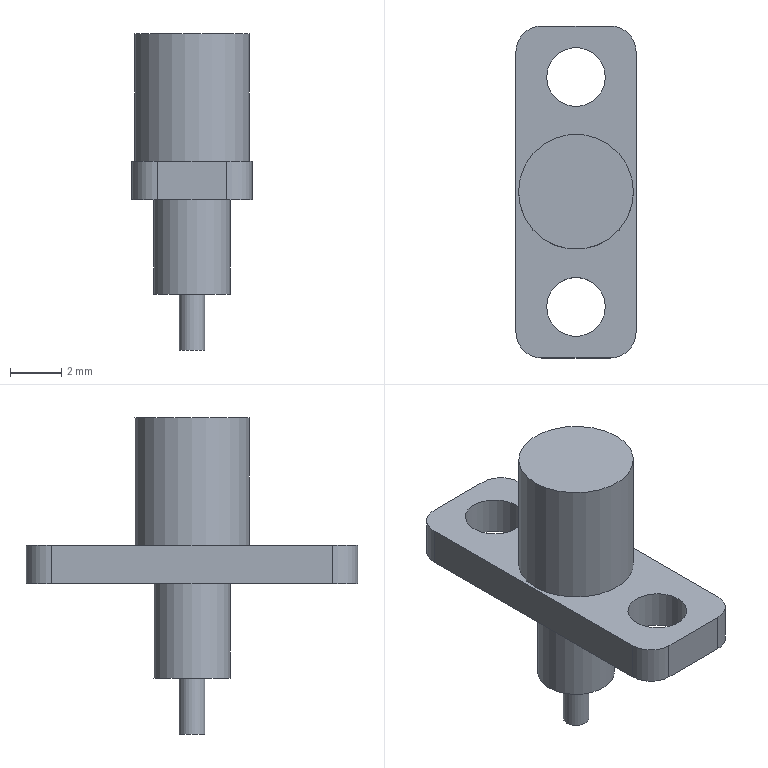Part | STEP file | MCX-KFD1 | 1 solid | 18 faces | box 4.7 x 13 x 12.4 mm | volume 185.301 mm3 | plane 9 | cylinder 9 | commonest cylinder face diameters 2 x4 2.3 x2 1 x1 3 x1 4.5 x1
STEP:
#1=CARTESIAN_POINT('',(0.,0.,0.));
#2=DIRECTION('',(0.,0.,1.));
#3=DIRECTION('',(1.,0.,0.));
#4=AXIS2_PLACEMENT_3D('',#1,#2,#3);
#5=CARTESIAN_POINT('',(-2.35,5.5,1.5));
#6=VERTEX_POINT('',#5);
#7=CARTESIAN_POINT('',(-2.35,-5.5,1.5));
#8=VERTEX_POINT('',#7);
#9=CARTESIAN_POINT('',(-2.35,6.5,1.5));
#10=DIRECTION('',(0.,-1.,0.));
#11=VECTOR('',#10,1.);
#12=LINE('',#9,#11);
#13=CARTESIAN_POINT('',(-2.35,6.5,1.5));
#14=DIRECTION('',(1.,0.,0.));
#15=DIRECTION('',(0.,0.,-1.));
#16=AXIS2_PLACEMENT_3D('',#13,#14,#15);
#17=PLANE('',#16);
#18=CARTESIAN_POINT('',(0.,0.));
#19=DIRECTION('',(0.,-1.));
#20=VECTOR('',#19,1.);
#21=LINE('',#18,#20);
#22=(GEOMETRIC_REPRESENTATION_CONTEXT(2)PARAMETRIC_REPRESENTATION_CONTEXT()REPRESENTATION_CONTEXT('',''));
#23=DEFINITIONAL_REPRESENTATION('',(#21),#22);
#24=PCURVE('',#17,#23);
#25=CARTESIAN_POINT('',(0.,4.5,1.5));
#26=DIRECTION('',(0.,0.,-1.));
#27=DIRECTION('',(-1.,0.,0.));
#28=AXIS2_PLACEMENT_3D('',#25,#26,#27);
#29=PLANE('',#28);
#30=CARTESIAN_POINT('',(2.35,2.));
#31=DIRECTION('',(0.,-1.));
#32=VECTOR('',#31,1.);
#33=LINE('',#30,#32);
#34=(GEOMETRIC_REPRESENTATION_CONTEXT(2)PARAMETRIC_REPRESENTATION_CONTEXT()REPRESENTATION_CONTEXT('',''));
#35=DEFINITIONAL_REPRESENTATION('',(#33),#34);
#36=PCURVE('',#29,#35);
#37=SURFACE_CURVE('',#12,(#24,#36),.PCURVE_S1.);
#38=EDGE_CURVE('',#6,#8,#37,.T.);
#39=ORIENTED_EDGE('',*,*,#38,.F.);
#40=CARTESIAN_POINT('',(-2.35,5.5,0.));
#41=VERTEX_POINT('',#40);
#42=CARTESIAN_POINT('',(-2.35,5.5,1.5));
#43=DIRECTION('',(0.,0.,-1.));
#44=VECTOR('',#43,1.);
#45=LINE('',#42,#44);
#46=CARTESIAN_POINT('',(0.,-1.));
#47=DIRECTION('',(1.,0.));
#48=VECTOR('',#47,1.);
#49=LINE('',#46,#48);
#50=(GEOMETRIC_REPRESENTATION_CONTEXT(2)PARAMETRIC_REPRESENTATION_CONTEXT()REPRESENTATION_CONTEXT('',''));
#51=DEFINITIONAL_REPRESENTATION('',(#49),#50);
#52=PCURVE('',#17,#51);
#53=CARTESIAN_POINT('',(-1.35,5.5,1.5));
#54=DIRECTION('',(0.,0.,-1.));
#55=DIRECTION('',(-1.,0.,0.));
#56=AXIS2_PLACEMENT_3D('',#53,#54,#55);
#57=CYLINDRICAL_SURFACE('',#56,1.);
#58=CARTESIAN_POINT('',(0.,0.));
#59=DIRECTION('',(0.,1.));
#60=VECTOR('',#59,1.);
#61=LINE('',#58,#60);
#62=(GEOMETRIC_REPRESENTATION_CONTEXT(2)PARAMETRIC_REPRESENTATION_CONTEXT()REPRESENTATION_CONTEXT('',''));
#63=DEFINITIONAL_REPRESENTATION('',(#61),#62);
#64=PCURVE('',#57,#63);
#65=SURFACE_CURVE('',#45,(#52,#64),.PCURVE_S1.);
#66=EDGE_CURVE('',#6,#41,#65,.T.);
#67=ORIENTED_EDGE('',*,*,#66,.T.);
#68=CARTESIAN_POINT('',(-2.35,-5.5,0.));
#69=VERTEX_POINT('',#68);
#70=CARTESIAN_POINT('',(-2.35,6.5,0.));
#71=DIRECTION('',(0.,-1.,0.));
#72=VECTOR('',#71,1.);
#73=LINE('',#70,#72);
#74=CARTESIAN_POINT('',(1.5,0.));
#75=DIRECTION('',(0.,-1.));
#76=VECTOR('',#75,1.);
#77=LINE('',#74,#76);
#78=(GEOMETRIC_REPRESENTATION_CONTEXT(2)PARAMETRIC_REPRESENTATION_CONTEXT()REPRESENTATION_CONTEXT('',''));
#79=DEFINITIONAL_REPRESENTATION('',(#77),#78);
#80=PCURVE('',#17,#79);
#81=CARTESIAN_POINT('',(0.,4.5,0.));
#82=DIRECTION('',(0.,0.,-1.));
#83=DIRECTION('',(-1.,0.,0.));
#84=AXIS2_PLACEMENT_3D('',#81,#82,#83);
#85=PLANE('',#84);
#86=CARTESIAN_POINT('',(2.35,2.));
#87=DIRECTION('',(0.,-1.));
#88=VECTOR('',#87,1.);
#89=LINE('',#86,#88);
#90=(GEOMETRIC_REPRESENTATION_CONTEXT(2)PARAMETRIC_REPRESENTATION_CONTEXT()REPRESENTATION_CONTEXT('',''));
#91=DEFINITIONAL_REPRESENTATION('',(#89),#90);
#92=PCURVE('',#85,#91);
#93=SURFACE_CURVE('',#73,(#80,#92),.PCURVE_S1.);
#94=EDGE_CURVE('',#41,#69,#93,.T.);
#95=ORIENTED_EDGE('',*,*,#94,.T.);
#96=CARTESIAN_POINT('',(-2.35,-5.5,1.5));
#97=DIRECTION('',(0.,0.,1.));
#98=VECTOR('',#97,1.);
#99=LINE('',#96,#98);
#100=CARTESIAN_POINT('',(0.,-12.));
#101=DIRECTION('',(-1.,0.));
#102=VECTOR('',#101,1.);
#103=LINE('',#100,#102);
#104=(GEOMETRIC_REPRESENTATION_CONTEXT(2)PARAMETRIC_REPRESENTATION_CONTEXT()REPRESENTATION_CONTEXT('',''));
#105=DEFINITIONAL_REPRESENTATION('',(#103),#104);
#106=PCURVE('',#17,#105);
#107=CARTESIAN_POINT('',(-1.35,-5.5,1.5));
#108=DIRECTION('',(0.,0.,-1.));
#109=DIRECTION('',(-1.,0.,0.));
#110=AXIS2_PLACEMENT_3D('',#107,#108,#109);
#111=CYLINDRICAL_SURFACE('',#110,1.);
#112=CARTESIAN_POINT('',(6.283,0.));
#113=DIRECTION('',(0.,-1.));
#114=VECTOR('',#113,1.);
#115=LINE('',#112,#114);
#116=(GEOMETRIC_REPRESENTATION_CONTEXT(2)PARAMETRIC_REPRESENTATION_CONTEXT()REPRESENTATION_CONTEXT('',''));
#117=DEFINITIONAL_REPRESENTATION('',(#115),#116);
#118=PCURVE('',#111,#117);
#119=SURFACE_CURVE('',#99,(#106,#118),.PCURVE_S1.);
#120=EDGE_CURVE('',#69,#8,#119,.T.);
#121=ORIENTED_EDGE('',*,*,#120,.T.);
#122=EDGE_LOOP('',(#39,#67,#95,#121));
#123=FACE_BOUND('',#122,.T.);
#124=ADVANCED_FACE('',(#123),#17,.F.);
#125=CARTESIAN_POINT('',(-1.35,-6.5,0.));
#126=VERTEX_POINT('',#125);
#127=CARTESIAN_POINT('',(1.35,-6.5,0.));
#128=VERTEX_POINT('',#127);
#129=CARTESIAN_POINT('',(-2.35,-6.5,0.));
#130=DIRECTION('',(1.,0.,0.));
#131=VECTOR('',#130,1.);
#132=LINE('',#129,#131);
#133=CARTESIAN_POINT('',(-2.35,-6.5,1.5));
#134=DIRECTION('',(0.,1.,0.));
#135=DIRECTION('',(0.,0.,1.));
#136=AXIS2_PLACEMENT_3D('',#133,#134,#135);
#137=PLANE('',#136);
#138=CARTESIAN_POINT('',(-1.5,0.));
#139=DIRECTION('',(0.,1.));
#140=VECTOR('',#139,1.);
#141=LINE('',#138,#140);
#142=(GEOMETRIC_REPRESENTATION_CONTEXT(2)PARAMETRIC_REPRESENTATION_CONTEXT()REPRESENTATION_CONTEXT('',''));
#143=DEFINITIONAL_REPRESENTATION('',(#141),#142);
#144=PCURVE('',#137,#143);
#145=CARTESIAN_POINT('',(2.35,-11.));
#146=DIRECTION('',(-1.,0.));
#147=VECTOR('',#146,1.);
#148=LINE('',#145,#147);
#149=(GEOMETRIC_REPRESENTATION_CONTEXT(2)PARAMETRIC_REPRESENTATION_CONTEXT()REPRESENTATION_CONTEXT('',''));
#150=DEFINITIONAL_REPRESENTATION('',(#148),#149);
#151=PCURVE('',#85,#150);
#152=SURFACE_CURVE('',#132,(#144,#151),.PCURVE_S1.);
#153=EDGE_CURVE('',#126,#128,#152,.T.);
#154=ORIENTED_EDGE('',*,*,#153,.T.);
#155=CARTESIAN_POINT('',(1.35,-6.5,1.5));
#156=VERTEX_POINT('',#155);
#157=CARTESIAN_POINT('',(1.35,-6.5,1.5));
#158=DIRECTION('',(0.,0.,1.));
#159=VECTOR('',#158,1.);
#160=LINE('',#157,#159);
#161=CARTESIAN_POINT('',(0.,3.7));
#162=DIRECTION('',(1.,0.));
#163=VECTOR('',#162,1.);
#164=LINE('',#161,#163);
#165=(GEOMETRIC_REPRESENTATION_CONTEXT(2)PARAMETRIC_REPRESENTATION_CONTEXT()REPRESENTATION_CONTEXT('',''));
#166=DEFINITIONAL_REPRESENTATION('',(#164),#165);
#167=PCURVE('',#137,#166);
#168=CARTESIAN_POINT('',(1.35,-5.5,1.5));
#169=DIRECTION('',(0.,0.,-1.));
#170=DIRECTION('',(-1.,0.,0.));
#171=AXIS2_PLACEMENT_3D('',#168,#169,#170);
#172=CYLINDRICAL_SURFACE('',#171,1.);
#173=CARTESIAN_POINT('',(4.712,0.));
#174=DIRECTION('',(0.,-1.));
#175=VECTOR('',#174,1.);
#176=LINE('',#173,#175);
#177=(GEOMETRIC_REPRESENTATION_CONTEXT(2)PARAMETRIC_REPRESENTATION_CONTEXT()REPRESENTATION_CONTEXT('',''));
#178=DEFINITIONAL_REPRESENTATION('',(#176),#177);
#179=PCURVE('',#172,#178);
#180=SURFACE_CURVE('',#160,(#167,#179),.PCURVE_S1.);
#181=EDGE_CURVE('',#128,#156,#180,.T.);
#182=ORIENTED_EDGE('',*,*,#181,.T.);
#183=CARTESIAN_POINT('',(-1.35,-6.5,1.5));
#184=VERTEX_POINT('',#183);
#185=CARTESIAN_POINT('',(-2.35,-6.5,1.5));
#186=DIRECTION('',(1.,0.,0.));
#187=VECTOR('',#186,1.);
#188=LINE('',#185,#187);
#189=CARTESIAN_POINT('',(0.,0.));
#190=DIRECTION('',(0.,1.));
#191=VECTOR('',#190,1.);
#192=LINE('',#189,#191);
#193=(GEOMETRIC_REPRESENTATION_CONTEXT(2)PARAMETRIC_REPRESENTATION_CONTEXT()REPRESENTATION_CONTEXT('',''));
#194=DEFINITIONAL_REPRESENTATION('',(#192),#193);
#195=PCURVE('',#137,#194);
#196=CARTESIAN_POINT('',(2.35,-11.));
#197=DIRECTION('',(-1.,0.));
#198=VECTOR('',#197,1.);
#199=LINE('',#196,#198);
#200=(GEOMETRIC_REPRESENTATION_CONTEXT(2)PARAMETRIC_REPRESENTATION_CONTEXT()REPRESENTATION_CONTEXT('',''));
#201=DEFINITIONAL_REPRESENTATION('',(#199),#200);
#202=PCURVE('',#29,#201);
#203=SURFACE_CURVE('',#188,(#195,#202),.PCURVE_S1.);
#204=EDGE_CURVE('',#184,#156,#203,.T.);
#205=ORIENTED_EDGE('',*,*,#204,.F.);
#206=CARTESIAN_POINT('',(-1.35,-6.5,1.5));
#207=DIRECTION('',(0.,0.,-1.));
#208=VECTOR('',#207,1.);
#209=LINE('',#206,#208);
#210=CARTESIAN_POINT('',(0.,1.));
#211=DIRECTION('',(-1.,0.));
#212=VECTOR('',#211,1.);
#213=LINE('',#210,#212);
#214=(GEOMETRIC_REPRESENTATION_CONTEXT(2)PARAMETRIC_REPRESENTATION_CONTEXT()REPRESENTATION_CONTEXT('',''));
#215=DEFINITIONAL_REPRESENTATION('',(#213),#214);
#216=PCURVE('',#137,#215);
#217=CARTESIAN_POINT('',(4.712,0.));
#218=DIRECTION('',(0.,1.));
#219=VECTOR('',#218,1.);
#220=LINE('',#217,#219);
#221=(GEOMETRIC_REPRESENTATION_CONTEXT(2)PARAMETRIC_REPRESENTATION_CONTEXT()REPRESENTATION_CONTEXT('',''));
#222=DEFINITIONAL_REPRESENTATION('',(#220),#221);
#223=PCURVE('',#111,#222);
#224=SURFACE_CURVE('',#209,(#216,#223),.PCURVE_S1.);
#225=EDGE_CURVE('',#184,#126,#224,.T.);
#226=ORIENTED_EDGE('',*,*,#225,.T.);
#227=EDGE_LOOP('',(#154,#182,#205,#226));
#228=FACE_BOUND('',#227,.T.);
#229=ADVANCED_FACE('',(#228),#137,.F.);
#230=CARTESIAN_POINT('',(2.35,-5.5,1.5));
#231=VERTEX_POINT('',#230);
#232=CARTESIAN_POINT('',(2.35,5.5,1.5));
#233=VERTEX_POINT('',#232);
#234=CARTESIAN_POINT('',(2.35,-6.5,1.5));
#235=DIRECTION('',(0.,1.,0.));
#236=VECTOR('',#235,1.);
#237=LINE('',#234,#236);
#238=CARTESIAN_POINT('',(2.35,-6.5,1.5));
#239=DIRECTION('',(-1.,0.,0.));
#240=DIRECTION('',(0.,0.,1.));
#241=AXIS2_PLACEMENT_3D('',#238,#239,#240);
#242=PLANE('',#241);
#243=CARTESIAN_POINT('',(0.,0.));
#244=DIRECTION('',(0.,1.));
#245=VECTOR('',#244,1.);
#246=LINE('',#243,#245);
#247=(GEOMETRIC_REPRESENTATION_CONTEXT(2)PARAMETRIC_REPRESENTATION_CONTEXT()REPRESENTATION_CONTEXT('',''));
#248=DEFINITIONAL_REPRESENTATION('',(#246),#247);
#249=PCURVE('',#242,#248);
#250=CARTESIAN_POINT('',(-2.35,-11.));
#251=DIRECTION('',(0.,1.));
#252=VECTOR('',#251,1.);
#253=LINE('',#250,#252);
#254=(GEOMETRIC_REPRESENTATION_CONTEXT(2)PARAMETRIC_REPRESENTATION_CONTEXT()REPRESENTATION_CONTEXT('',''));
#255=DEFINITIONAL_REPRESENTATION('',(#253),#254);
#256=PCURVE('',#29,#255);
#257=SURFACE_CURVE('',#237,(#249,#256),.PCURVE_S1.);
#258=EDGE_CURVE('',#231,#233,#257,.T.);
#259=ORIENTED_EDGE('',*,*,#258,.F.);
#260=CARTESIAN_POINT('',(2.35,-5.5,0.));
#261=VERTEX_POINT('',#260);
#262=CARTESIAN_POINT('',(2.35,-5.5,1.5));
#263=DIRECTION('',(0.,0.,-1.));
#264=VECTOR('',#263,1.);
#265=LINE('',#262,#264);
#266=CARTESIAN_POINT('',(0.,1.));
#267=DIRECTION('',(-1.,0.));
#268=VECTOR('',#267,1.);
#269=LINE('',#266,#268);
#270=(GEOMETRIC_REPRESENTATION_CONTEXT(2)PARAMETRIC_REPRESENTATION_CONTEXT()REPRESENTATION_CONTEXT('',''));
#271=DEFINITIONAL_REPRESENTATION('',(#269),#270);
#272=PCURVE('',#242,#271);
#273=CARTESIAN_POINT('',(3.142,0.));
#274=DIRECTION('',(0.,1.));
#275=VECTOR('',#274,1.);
#276=LINE('',#273,#275);
#277=(GEOMETRIC_REPRESENTATION_CONTEXT(2)PARAMETRIC_REPRESENTATION_CONTEXT()REPRESENTATION_CONTEXT('',''));
#278=DEFINITIONAL_REPRESENTATION('',(#276),#277);
#279=PCURVE('',#172,#278);
#280=SURFACE_CURVE('',#265,(#272,#279),.PCURVE_S1.);
#281=EDGE_CURVE('',#231,#261,#280,.T.);
#282=ORIENTED_EDGE('',*,*,#281,.T.);
#283=CARTESIAN_POINT('',(2.35,5.5,0.));
#284=VERTEX_POINT('',#283);
#285=CARTESIAN_POINT('',(2.35,-6.5,0.));
#286=DIRECTION('',(0.,1.,0.));
#287=VECTOR('',#286,1.);
#288=LINE('',#285,#287);
#289=CARTESIAN_POINT('',(-1.5,0.));
#290=DIRECTION('',(0.,1.));
#291=VECTOR('',#290,1.);
#292=LINE('',#289,#291);
#293=(GEOMETRIC_REPRESENTATION_CONTEXT(2)PARAMETRIC_REPRESENTATION_CONTEXT()REPRESENTATION_CONTEXT('',''));
#294=DEFINITIONAL_REPRESENTATION('',(#292),#293);
#295=PCURVE('',#242,#294);
#296=CARTESIAN_POINT('',(-2.35,-11.));
#297=DIRECTION('',(0.,1.));
#298=VECTOR('',#297,1.);
#299=LINE('',#296,#298);
#300=(GEOMETRIC_REPRESENTATION_CONTEXT(2)PARAMETRIC_REPRESENTATION_CONTEXT()REPRESENTATION_CONTEXT('',''));
#301=DEFINITIONAL_REPRESENTATION('',(#299),#300);
#302=PCURVE('',#85,#301);
#303=SURFACE_CURVE('',#288,(#295,#302),.PCURVE_S1.);
#304=EDGE_CURVE('',#261,#284,#303,.T.);
#305=ORIENTED_EDGE('',*,*,#304,.T.);
#306=CARTESIAN_POINT('',(2.35,5.5,1.5));
#307=DIRECTION('',(0.,0.,1.));
#308=VECTOR('',#307,1.);
#309=LINE('',#306,#308);
#310=CARTESIAN_POINT('',(0.,12.));
#311=DIRECTION('',(1.,0.));
#312=VECTOR('',#311,1.);
#313=LINE('',#310,#312);
#314=(GEOMETRIC_REPRESENTATION_CONTEXT(2)PARAMETRIC_REPRESENTATION_CONTEXT()REPRESENTATION_CONTEXT('',''));
#315=DEFINITIONAL_REPRESENTATION('',(#313),#314);
#316=PCURVE('',#242,#315);
#317=CARTESIAN_POINT('',(1.35,5.5,1.5));
#318=DIRECTION('',(0.,0.,-1.));
#319=DIRECTION('',(-1.,0.,0.));
#320=AXIS2_PLACEMENT_3D('',#317,#318,#319);
#321=CYLINDRICAL_SURFACE('',#320,1.);
#322=CARTESIAN_POINT('',(3.142,0.));
#323=DIRECTION('',(0.,-1.));
#324=VECTOR('',#323,1.);
#325=LINE('',#322,#324);
#326=(GEOMETRIC_REPRESENTATION_CONTEXT(2)PARAMETRIC_REPRESENTATION_CONTEXT()REPRESENTATION_CONTEXT('',''));
#327=DEFINITIONAL_REPRESENTATION('',(#325),#326);
#328=PCURVE('',#321,#327);
#329=SURFACE_CURVE('',#309,(#316,#328),.PCURVE_S1.);
#330=EDGE_CURVE('',#284,#233,#329,.T.);
#331=ORIENTED_EDGE('',*,*,#330,.T.);
#332=EDGE_LOOP('',(#259,#282,#305,#331));
#333=FACE_BOUND('',#332,.T.);
#334=ADVANCED_FACE('',(#333),#242,.F.);
#335=CARTESIAN_POINT('',(1.15,4.5,1.5));
#336=VERTEX_POINT('',#335);
#337=CARTESIAN_POINT('',(0.,4.5,1.5));
#338=DIRECTION('',(0.,0.,-1.));
#339=DIRECTION('',(1.,0.,0.));
#340=AXIS2_PLACEMENT_3D('',#337,#338,#339);
#341=CIRCLE('',#340,1.15);
#342=CARTESIAN_POINT('',(0.,4.5,1.5));
#343=DIRECTION('',(0.,0.,-1.));
#344=DIRECTION('',(-1.,0.,0.));
#345=AXIS2_PLACEMENT_3D('',#342,#343,#344);
#346=CYLINDRICAL_SURFACE('',#345,1.15);
#347=CARTESIAN_POINT('',(3.142,0.));
#348=DIRECTION('',(1.,0.));
#349=VECTOR('',#348,1.);
#350=LINE('',#347,#349);
#351=(GEOMETRIC_REPRESENTATION_CONTEXT(2)PARAMETRIC_REPRESENTATION_CONTEXT()REPRESENTATION_CONTEXT('',''));
#352=DEFINITIONAL_REPRESENTATION('',(#350),#351);
#353=PCURVE('',#346,#352);
#354=CARTESIAN_POINT('',(0.,0.));
#355=DIRECTION('',(-1.,0.));
#356=AXIS2_PLACEMENT_2D('',#354,#355);
#357=CIRCLE('',#356,1.15);
#358=(GEOMETRIC_REPRESENTATION_CONTEXT(2)PARAMETRIC_REPRESENTATION_CONTEXT()REPRESENTATION_CONTEXT('',''));
#359=DEFINITIONAL_REPRESENTATION('',(#357),#358);
#360=PCURVE('',#29,#359);
#361=SURFACE_CURVE('',#341,(#353,#360),.PCURVE_S1.);
#362=EDGE_CURVE('',#336,#336,#361,.T.);
#363=ORIENTED_EDGE('',*,*,#362,.T.);
#364=CARTESIAN_POINT('',(1.15,4.5,0.));
#365=VERTEX_POINT('',#364);
#366=CARTESIAN_POINT('',(1.15,4.5,1.5));
#367=CARTESIAN_POINT('',(1.15,4.5,0.));
#368=B_SPLINE_CURVE_WITH_KNOTS('',1,(#366,#367),.UNSPECIFIED.,.F.,.F.,(2,2),(0.,1.5),.PIECEWISE_BEZIER_KNOTS.);
#369=CARTESIAN_POINT('',(9.425,0.));
#370=DIRECTION('',(0.,1.));
#371=VECTOR('',#370,1.);
#372=LINE('',#369,#371);
#373=(GEOMETRIC_REPRESENTATION_CONTEXT(2)PARAMETRIC_REPRESENTATION_CONTEXT()REPRESENTATION_CONTEXT('',''));
#374=DEFINITIONAL_REPRESENTATION('',(#372),#373);
#375=PCURVE('',#346,#374);
#376=CARTESIAN_POINT('',(3.142,0.));
#377=DIRECTION('',(0.,1.));
#378=VECTOR('',#377,1.);
#379=LINE('',#376,#378);
#380=(GEOMETRIC_REPRESENTATION_CONTEXT(2)PARAMETRIC_REPRESENTATION_CONTEXT()REPRESENTATION_CONTEXT('',''));
#381=DEFINITIONAL_REPRESENTATION('',(#379),#380);
#382=PCURVE('',#346,#381);
#383=SEAM_CURVE('',#368,(#375,#382),.PCURVE_S1.);
#384=EDGE_CURVE('',#336,#365,#383,.T.);
#385=ORIENTED_EDGE('',*,*,#384,.T.);
#386=CARTESIAN_POINT('',(0.,4.5,0.));
#387=DIRECTION('',(0.,0.,-1.));
#388=DIRECTION('',(1.,0.,0.));
#389=AXIS2_PLACEMENT_3D('',#386,#387,#388);
#390=CIRCLE('',#389,1.15);
#391=CARTESIAN_POINT('',(3.142,1.5));
#392=DIRECTION('',(1.,0.));
#393=VECTOR('',#392,1.);
#394=LINE('',#391,#393);
#395=(GEOMETRIC_REPRESENTATION_CONTEXT(2)PARAMETRIC_REPRESENTATION_CONTEXT()REPRESENTATION_CONTEXT('',''));
#396=DEFINITIONAL_REPRESENTATION('',(#394),#395);
#397=PCURVE('',#346,#396);
#398=CARTESIAN_POINT('',(0.,0.));
#399=DIRECTION('',(-1.,0.));
#400=AXIS2_PLACEMENT_2D('',#398,#399);
#401=CIRCLE('',#400,1.15);
#402=(GEOMETRIC_REPRESENTATION_CONTEXT(2)PARAMETRIC_REPRESENTATION_CONTEXT()REPRESENTATION_CONTEXT('',''));
#403=DEFINITIONAL_REPRESENTATION('',(#401),#402);
#404=PCURVE('',#85,#403);
#405=SURFACE_CURVE('',#390,(#397,#404),.PCURVE_S1.);
#406=EDGE_CURVE('',#365,#365,#405,.T.);
#407=ORIENTED_EDGE('',*,*,#406,.F.);
#408=ORIENTED_EDGE('',*,*,#384,.F.);
#409=EDGE_LOOP('',(#363,#385,#407,#408));
#410=FACE_BOUND('',#409,.F.);
#411=ADVANCED_FACE('',(#410),#346,.F.);
#412=CARTESIAN_POINT('',(1.35,6.5,0.));
#413=VERTEX_POINT('',#412);
#414=CARTESIAN_POINT('',(-1.35,6.5,0.));
#415=VERTEX_POINT('',#414);
#416=CARTESIAN_POINT('',(2.35,6.5,0.));
#417=DIRECTION('',(-1.,0.,0.));
#418=VECTOR('',#417,1.);
#419=LINE('',#416,#418);
#420=CARTESIAN_POINT('',(2.35,6.5,1.5));
#421=DIRECTION('',(0.,-1.,0.));
#422=DIRECTION('',(0.,0.,-1.));
#423=AXIS2_PLACEMENT_3D('',#420,#421,#422);
#424=PLANE('',#423);
#425=CARTESIAN_POINT('',(1.5,0.));
#426=DIRECTION('',(0.,-1.));
#427=VECTOR('',#426,1.);
#428=LINE('',#425,#427);
#429=(GEOMETRIC_REPRESENTATION_CONTEXT(2)PARAMETRIC_REPRESENTATION_CONTEXT()REPRESENTATION_CONTEXT('',''));
#430=DEFINITIONAL_REPRESENTATION('',(#428),#429);
#431=PCURVE('',#424,#430);
#432=CARTESIAN_POINT('',(-2.35,2.));
#433=DIRECTION('',(1.,0.));
#434=VECTOR('',#433,1.);
#435=LINE('',#432,#434);
#436=(GEOMETRIC_REPRESENTATION_CONTEXT(2)PARAMETRIC_REPRESENTATION_CONTEXT()REPRESENTATION_CONTEXT('',''));
#437=DEFINITIONAL_REPRESENTATION('',(#435),#436);
#438=PCURVE('',#85,#437);
#439=SURFACE_CURVE('',#419,(#431,#438),.PCURVE_S1.);
#440=EDGE_CURVE('',#413,#415,#439,.T.);
#441=ORIENTED_EDGE('',*,*,#440,.T.);
#442=CARTESIAN_POINT('',(-1.35,6.5,1.5));
#443=VERTEX_POINT('',#442);
#444=CARTESIAN_POINT('',(-1.35,6.5,1.5));
#445=DIRECTION('',(0.,0.,1.));
#446=VECTOR('',#445,1.);
#447=LINE('',#444,#446);
#448=CARTESIAN_POINT('',(0.,-3.7));
#449=DIRECTION('',(-1.,0.));
#450=VECTOR('',#449,1.);
#451=LINE('',#448,#450);
#452=(GEOMETRIC_REPRESENTATION_CONTEXT(2)PARAMETRIC_REPRESENTATION_CONTEXT()REPRESENTATION_CONTEXT('',''));
#453=DEFINITIONAL_REPRESENTATION('',(#451),#452);
#454=PCURVE('',#424,#453);
#455=CARTESIAN_POINT('',(1.571,0.));
#456=DIRECTION('',(0.,-1.));
#457=VECTOR('',#456,1.);
#458=LINE('',#455,#457);
#459=(GEOMETRIC_REPRESENTATION_CONTEXT(2)PARAMETRIC_REPRESENTATION_CONTEXT()REPRESENTATION_CONTEXT('',''));
#460=DEFINITIONAL_REPRESENTATION('',(#458),#459);
#461=PCURVE('',#57,#460);
#462=SURFACE_CURVE('',#447,(#454,#461),.PCURVE_S1.);
#463=EDGE_CURVE('',#415,#443,#462,.T.);
#464=ORIENTED_EDGE('',*,*,#463,.T.);
#465=CARTESIAN_POINT('',(1.35,6.5,1.5));
#466=VERTEX_POINT('',#465);
#467=CARTESIAN_POINT('',(2.35,6.5,1.5));
#468=DIRECTION('',(-1.,0.,0.));
#469=VECTOR('',#468,1.);
#470=LINE('',#467,#469);
#471=CARTESIAN_POINT('',(0.,0.));
#472=DIRECTION('',(0.,-1.));
#473=VECTOR('',#472,1.);
#474=LINE('',#471,#473);
#475=(GEOMETRIC_REPRESENTATION_CONTEXT(2)PARAMETRIC_REPRESENTATION_CONTEXT()REPRESENTATION_CONTEXT('',''));
#476=DEFINITIONAL_REPRESENTATION('',(#474),#475);
#477=PCURVE('',#424,#476);
#478=CARTESIAN_POINT('',(-2.35,2.));
#479=DIRECTION('',(1.,0.));
#480=VECTOR('',#479,1.);
#481=LINE('',#478,#480);
#482=(GEOMETRIC_REPRESENTATION_CONTEXT(2)PARAMETRIC_REPRESENTATION_CONTEXT()REPRESENTATION_CONTEXT('',''));
#483=DEFINITIONAL_REPRESENTATION('',(#481),#482);
#484=PCURVE('',#29,#483);
#485=SURFACE_CURVE('',#470,(#477,#484),.PCURVE_S1.);
#486=EDGE_CURVE('',#466,#443,#485,.T.);
#487=ORIENTED_EDGE('',*,*,#486,.F.);
#488=CARTESIAN_POINT('',(1.35,6.5,1.5));
#489=DIRECTION('',(0.,0.,-1.));
#490=VECTOR('',#489,1.);
#491=LINE('',#488,#490);
#492=CARTESIAN_POINT('',(0.,-1.));
#493=DIRECTION('',(1.,0.));
#494=VECTOR('',#493,1.);
#495=LINE('',#492,#494);
#496=(GEOMETRIC_REPRESENTATION_CONTEXT(2)PARAMETRIC_REPRESENTATION_CONTEXT()REPRESENTATION_CONTEXT('',''));
#497=DEFINITIONAL_REPRESENTATION('',(#495),#496);
#498=PCURVE('',#424,#497);
#499=CARTESIAN_POINT('',(1.571,0.));
#500=DIRECTION('',(0.,1.));
#501=VECTOR('',#500,1.);
#502=LINE('',#499,#501);
#503=(GEOMETRIC_REPRESENTATION_CONTEXT(2)PARAMETRIC_REPRESENTATION_CONTEXT()REPRESENTATION_CONTEXT('',''));
#504=DEFINITIONAL_REPRESENTATION('',(#502),#503);
#505=PCURVE('',#321,#504);
#506=SURFACE_CURVE('',#491,(#498,#505),.PCURVE_S1.);
#507=EDGE_CURVE('',#466,#413,#506,.T.);
#508=ORIENTED_EDGE('',*,*,#507,.T.);
#509=EDGE_LOOP('',(#441,#464,#487,#508));
#510=FACE_BOUND('',#509,.T.);
#511=ADVANCED_FACE('',(#510),#424,.F.);
#512=CARTESIAN_POINT('',(1.15,-4.5,1.5));
#513=VERTEX_POINT('',#512);
#514=CARTESIAN_POINT('',(0.,-4.5,1.5));
#515=DIRECTION('',(0.,0.,1.));
#516=DIRECTION('',(1.,0.,0.));
#517=AXIS2_PLACEMENT_3D('',#514,#515,#516);
#518=CIRCLE('',#517,1.15);
#519=CARTESIAN_POINT('',(0.,-4.5,1.5));
#520=DIRECTION('',(0.,0.,-1.));
#521=DIRECTION('',(-1.,0.,0.));
#522=AXIS2_PLACEMENT_3D('',#519,#520,#521);
#523=CYLINDRICAL_SURFACE('',#522,1.15);
#524=CARTESIAN_POINT('',(9.425,0.));
#525=DIRECTION('',(-1.,0.));
#526=VECTOR('',#525,1.);
#527=LINE('',#524,#526);
#528=(GEOMETRIC_REPRESENTATION_CONTEXT(2)PARAMETRIC_REPRESENTATION_CONTEXT()REPRESENTATION_CONTEXT('',''));
#529=DEFINITIONAL_REPRESENTATION('',(#527),#528);
#530=PCURVE('',#523,#529);
#531=CARTESIAN_POINT('',(-1.15,-9.));
#532=CARTESIAN_POINT('',(-1.15,-7.008));
#533=CARTESIAN_POINT('',(0.575,-8.004));
#534=CARTESIAN_POINT('',(2.3,-9.));
#535=CARTESIAN_POINT('',(0.575,-9.996));
#536=CARTESIAN_POINT('',(-1.15,-10.992));
#537=CARTESIAN_POINT('',(-1.15,-9.));
#538=(BOUNDED_CURVE()B_SPLINE_CURVE(2,(#531,#532,#533,#534,#535,#536,#537),.UNSPECIFIED.,.T.,.F.)B_SPLINE_CURVE_WITH_KNOTS((1,2,2,2,2,1),(-2.094,0.,2.094,4.189,6.283,8.378),.UNSPECIFIED.)CURVE()GEOMETRIC_REPRESENTATION_ITEM()RATIONAL_B_SPLINE_CURVE((1.,0.5,1.,0.5,1.,0.5,1.))REPRESENTATION_ITEM(''));
#539=(GEOMETRIC_REPRESENTATION_CONTEXT(2)PARAMETRIC_REPRESENTATION_CONTEXT()REPRESENTATION_CONTEXT('',''));
#540=DEFINITIONAL_REPRESENTATION('',(#538),#539);
#541=PCURVE('',#29,#540);
#542=SURFACE_CURVE('',#518,(#530,#541),.PCURVE_S1.);
#543=EDGE_CURVE('',#513,#513,#542,.T.);
#544=ORIENTED_EDGE('',*,*,#543,.F.);
#545=CARTESIAN_POINT('',(1.15,-4.5,0.));
#546=VERTEX_POINT('',#545);
#547=CARTESIAN_POINT('',(1.15,-4.5,1.5));
#548=CARTESIAN_POINT('',(1.15,-4.5,0.));
#549=B_SPLINE_CURVE_WITH_KNOTS('',1,(#547,#548),.UNSPECIFIED.,.F.,.F.,(2,2),(0.,1.5),.PIECEWISE_BEZIER_KNOTS.);
#550=CARTESIAN_POINT('',(9.425,0.));
#551=DIRECTION('',(0.,1.));
#552=VECTOR('',#551,1.);
#553=LINE('',#550,#552);
#554=(GEOMETRIC_REPRESENTATION_CONTEXT(2)PARAMETRIC_REPRESENTATION_CONTEXT()REPRESENTATION_CONTEXT('',''));
#555=DEFINITIONAL_REPRESENTATION('',(#553),#554);
#556=PCURVE('',#523,#555);
#557=CARTESIAN_POINT('',(3.142,0.));
#558=DIRECTION('',(0.,1.));
#559=VECTOR('',#558,1.);
#560=LINE('',#557,#559);
#561=(GEOMETRIC_REPRESENTATION_CONTEXT(2)PARAMETRIC_REPRESENTATION_CONTEXT()REPRESENTATION_CONTEXT('',''));
#562=DEFINITIONAL_REPRESENTATION('',(#560),#561);
#563=PCURVE('',#523,#562);
#564=SEAM_CURVE('',#549,(#556,#563),.PCURVE_S1.);
#565=EDGE_CURVE('',#513,#546,#564,.T.);
#566=ORIENTED_EDGE('',*,*,#565,.T.);
#567=CARTESIAN_POINT('',(0.,-4.5,0.));
#568=DIRECTION('',(0.,0.,1.));
#569=DIRECTION('',(1.,0.,0.));
#570=AXIS2_PLACEMENT_3D('',#567,#568,#569);
#571=CIRCLE('',#570,1.15);
#572=CARTESIAN_POINT('',(9.425,1.5));
#573=DIRECTION('',(-1.,0.));
#574=VECTOR('',#573,1.);
#575=LINE('',#572,#574);
#576=(GEOMETRIC_REPRESENTATION_CONTEXT(2)PARAMETRIC_REPRESENTATION_CONTEXT()REPRESENTATION_CONTEXT('',''));
#577=DEFINITIONAL_REPRESENTATION('',(#575),#576);
#578=PCURVE('',#523,#577);
#579=CARTESIAN_POINT('',(-1.15,-9.));
#580=CARTESIAN_POINT('',(-1.15,-7.008));
#581=CARTESIAN_POINT('',(0.575,-8.004));
#582=CARTESIAN_POINT('',(2.3,-9.));
#583=CARTESIAN_POINT('',(0.575,-9.996));
#584=CARTESIAN_POINT('',(-1.15,-10.992));
#585=CARTESIAN_POINT('',(-1.15,-9.));
#586=(BOUNDED_CURVE()B_SPLINE_CURVE(2,(#579,#580,#581,#582,#583,#584,#585),.UNSPECIFIED.,.T.,.F.)B_SPLINE_CURVE_WITH_KNOTS((1,2,2,2,2,1),(-2.094,0.,2.094,4.189,6.283,8.378),.UNSPECIFIED.)CURVE()GEOMETRIC_REPRESENTATION_ITEM()RATIONAL_B_SPLINE_CURVE((1.,0.5,1.,0.5,1.,0.5,1.))REPRESENTATION_ITEM(''));
#587=(GEOMETRIC_REPRESENTATION_CONTEXT(2)PARAMETRIC_REPRESENTATION_CONTEXT()REPRESENTATION_CONTEXT('',''));
#588=DEFINITIONAL_REPRESENTATION('',(#586),#587);
#589=PCURVE('',#85,#588);
#590=SURFACE_CURVE('',#571,(#578,#589),.PCURVE_S1.);
#591=EDGE_CURVE('',#546,#546,#590,.T.);
#592=ORIENTED_EDGE('',*,*,#591,.T.);
#593=ORIENTED_EDGE('',*,*,#565,.F.);
#594=EDGE_LOOP('',(#544,#566,#592,#593));
#595=FACE_BOUND('',#594,.F.);
#596=ADVANCED_FACE('',(#595),#523,.F.);
#597=CARTESIAN_POINT('',(-2.25,0.,1.5));
#598=VERTEX_POINT('',#597);
#599=CARTESIAN_POINT('',(0.,0.,1.5));
#600=DIRECTION('',(0.,0.,1.));
#601=DIRECTION('',(-1.,0.,0.));
#602=AXIS2_PLACEMENT_3D('',#599,#600,#601);
#603=CIRCLE('',#602,2.25);
#604=CARTESIAN_POINT('',(2.25,-4.5));
#605=CARTESIAN_POINT('',(2.25,-8.397));
#606=CARTESIAN_POINT('',(-1.125,-6.449));
#607=CARTESIAN_POINT('',(-4.5,-4.5));
#608=CARTESIAN_POINT('',(-1.125,-2.551));
#609=CARTESIAN_POINT('',(2.25,-0.6029));
#610=CARTESIAN_POINT('',(2.25,-4.5));
#611=(BOUNDED_CURVE()B_SPLINE_CURVE(2,(#604,#605,#606,#607,#608,#609,#610),.UNSPECIFIED.,.T.,.F.)B_SPLINE_CURVE_WITH_KNOTS((1,2,2,2,2,1),(-2.094,0.,2.094,4.189,6.283,8.378),.UNSPECIFIED.)CURVE()GEOMETRIC_REPRESENTATION_ITEM()RATIONAL_B_SPLINE_CURVE((1.,0.5,1.,0.5,1.,0.5,1.))REPRESENTATION_ITEM(''));
#612=(GEOMETRIC_REPRESENTATION_CONTEXT(2)PARAMETRIC_REPRESENTATION_CONTEXT()REPRESENTATION_CONTEXT('',''));
#613=DEFINITIONAL_REPRESENTATION('',(#611),#612);
#614=PCURVE('',#29,#613);
#615=CARTESIAN_POINT('',(0.,0.,6.5));
#616=DIRECTION('',(0.,0.,-1.));
#617=DIRECTION('',(-1.,0.,0.));
#618=AXIS2_PLACEMENT_3D('',#615,#616,#617);
#619=CYLINDRICAL_SURFACE('',#618,2.25);
#620=CARTESIAN_POINT('',(6.283,5.));
#621=DIRECTION('',(-1.,0.));
#622=VECTOR('',#621,1.);
#623=LINE('',#620,#622);
#624=(GEOMETRIC_REPRESENTATION_CONTEXT(2)PARAMETRIC_REPRESENTATION_CONTEXT()REPRESENTATION_CONTEXT('',''));
#625=DEFINITIONAL_REPRESENTATION('',(#623),#624);
#626=PCURVE('',#619,#625);
#627=SURFACE_CURVE('',#603,(#614,#626),.PCURVE_S1.);
#628=EDGE_CURVE('',#598,#598,#627,.T.);
#629=ORIENTED_EDGE('',*,*,#628,.F.);
#630=EDGE_LOOP('',(#629));
#631=FACE_BOUND('',#630,.T.);
#632=ORIENTED_EDGE('',*,*,#486,.T.);
#633=CARTESIAN_POINT('',(-1.35,5.5,1.5));
#634=DIRECTION('',(0.,0.,1.));
#635=DIRECTION('',(-1.,0.,0.));
#636=AXIS2_PLACEMENT_3D('',#633,#634,#635);
#637=CIRCLE('',#636,1.);
#638=CARTESIAN_POINT('',(2.35,1.));
#639=CARTESIAN_POINT('',(2.35,-0.7321));
#640=CARTESIAN_POINT('',(0.85,0.134));
#641=CARTESIAN_POINT('',(-0.65,1.));
#642=CARTESIAN_POINT('',(0.85,1.866));
#643=CARTESIAN_POINT('',(2.35,2.732));
#644=CARTESIAN_POINT('',(2.35,1.));
#645=(BOUNDED_CURVE()B_SPLINE_CURVE(2,(#638,#639,#640,#641,#642,#643,#644),.UNSPECIFIED.,.T.,.F.)B_SPLINE_CURVE_WITH_KNOTS((1,2,2,2,2,1),(-2.094,0.,2.094,4.189,6.283,8.378),.UNSPECIFIED.)CURVE()GEOMETRIC_REPRESENTATION_ITEM()RATIONAL_B_SPLINE_CURVE((1.,0.5,1.,0.5,1.,0.5,1.))REPRESENTATION_ITEM(''));
#646=(GEOMETRIC_REPRESENTATION_CONTEXT(2)PARAMETRIC_REPRESENTATION_CONTEXT()REPRESENTATION_CONTEXT('',''));
#647=DEFINITIONAL_REPRESENTATION('',(#645),#646);
#648=PCURVE('',#29,#647);
#649=CARTESIAN_POINT('',(6.283,0.));
#650=DIRECTION('',(-1.,0.));
#651=VECTOR('',#650,1.);
#652=LINE('',#649,#651);
#653=(GEOMETRIC_REPRESENTATION_CONTEXT(2)PARAMETRIC_REPRESENTATION_CONTEXT()REPRESENTATION_CONTEXT('',''));
#654=DEFINITIONAL_REPRESENTATION('',(#652),#653);
#655=PCURVE('',#57,#654);
#656=SURFACE_CURVE('',#637,(#648,#655),.PCURVE_S1.);
#657=EDGE_CURVE('',#443,#6,#656,.T.);
#658=ORIENTED_EDGE('',*,*,#657,.T.);
#659=ORIENTED_EDGE('',*,*,#38,.T.);
#660=CARTESIAN_POINT('',(-1.35,-5.5,1.5));
#661=DIRECTION('',(0.,0.,1.));
#662=DIRECTION('',(-1.,0.,0.));
#663=AXIS2_PLACEMENT_3D('',#660,#661,#662);
#664=CIRCLE('',#663,1.);
#665=CARTESIAN_POINT('',(2.35,-10.));
#666=CARTESIAN_POINT('',(2.35,-11.732));
#667=CARTESIAN_POINT('',(0.85,-10.866));
#668=CARTESIAN_POINT('',(-0.65,-10.));
#669=CARTESIAN_POINT('',(0.85,-9.134));
#670=CARTESIAN_POINT('',(2.35,-8.268));
#671=CARTESIAN_POINT('',(2.35,-10.));
#672=(BOUNDED_CURVE()B_SPLINE_CURVE(2,(#665,#666,#667,#668,#669,#670,#671),.UNSPECIFIED.,.T.,.F.)B_SPLINE_CURVE_WITH_KNOTS((1,2,2,2,2,1),(-2.094,0.,2.094,4.189,6.283,8.378),.UNSPECIFIED.)CURVE()GEOMETRIC_REPRESENTATION_ITEM()RATIONAL_B_SPLINE_CURVE((1.,0.5,1.,0.5,1.,0.5,1.))REPRESENTATION_ITEM(''));
#673=(GEOMETRIC_REPRESENTATION_CONTEXT(2)PARAMETRIC_REPRESENTATION_CONTEXT()REPRESENTATION_CONTEXT('',''));
#674=DEFINITIONAL_REPRESENTATION('',(#672),#673);
#675=PCURVE('',#29,#674);
#676=CARTESIAN_POINT('',(6.283,0.));
#677=DIRECTION('',(-1.,0.));
#678=VECTOR('',#677,1.);
#679=LINE('',#676,#678);
#680=(GEOMETRIC_REPRESENTATION_CONTEXT(2)PARAMETRIC_REPRESENTATION_CONTEXT()REPRESENTATION_CONTEXT('',''));
#681=DEFINITIONAL_REPRESENTATION('',(#679),#680);
#682=PCURVE('',#111,#681);
#683=SURFACE_CURVE('',#664,(#675,#682),.PCURVE_S1.);
#684=EDGE_CURVE('',#8,#184,#683,.T.);
#685=ORIENTED_EDGE('',*,*,#684,.T.);
#686=ORIENTED_EDGE('',*,*,#204,.T.);
#687=CARTESIAN_POINT('',(1.35,-5.5,1.5));
#688=DIRECTION('',(0.,0.,1.));
#689=DIRECTION('',(-1.,0.,0.));
#690=AXIS2_PLACEMENT_3D('',#687,#688,#689);
#691=CIRCLE('',#690,1.);
#692=CARTESIAN_POINT('',(-0.35,-10.));
#693=CARTESIAN_POINT('',(-0.35,-11.732));
#694=CARTESIAN_POINT('',(-1.85,-10.866));
#695=CARTESIAN_POINT('',(-3.35,-10.));
#696=CARTESIAN_POINT('',(-1.85,-9.134));
#697=CARTESIAN_POINT('',(-0.35,-8.268));
#698=CARTESIAN_POINT('',(-0.35,-10.));
#699=(BOUNDED_CURVE()B_SPLINE_CURVE(2,(#692,#693,#694,#695,#696,#697,#698),.UNSPECIFIED.,.T.,.F.)B_SPLINE_CURVE_WITH_KNOTS((1,2,2,2,2,1),(-2.094,0.,2.094,4.189,6.283,8.378),.UNSPECIFIED.)CURVE()GEOMETRIC_REPRESENTATION_ITEM()RATIONAL_B_SPLINE_CURVE((1.,0.5,1.,0.5,1.,0.5,1.))REPRESENTATION_ITEM(''));
#700=(GEOMETRIC_REPRESENTATION_CONTEXT(2)PARAMETRIC_REPRESENTATION_CONTEXT()REPRESENTATION_CONTEXT('',''));
#701=DEFINITIONAL_REPRESENTATION('',(#699),#700);
#702=PCURVE('',#29,#701);
#703=CARTESIAN_POINT('',(6.283,0.));
#704=DIRECTION('',(-1.,0.));
#705=VECTOR('',#704,1.);
#706=LINE('',#703,#705);
#707=(GEOMETRIC_REPRESENTATION_CONTEXT(2)PARAMETRIC_REPRESENTATION_CONTEXT()REPRESENTATION_CONTEXT('',''));
#708=DEFINITIONAL_REPRESENTATION('',(#706),#707);
#709=PCURVE('',#172,#708);
#710=SURFACE_CURVE('',#691,(#702,#709),.PCURVE_S1.);
#711=EDGE_CURVE('',#156,#231,#710,.T.);
#712=ORIENTED_EDGE('',*,*,#711,.T.);
#713=ORIENTED_EDGE('',*,*,#258,.T.);
#714=CARTESIAN_POINT('',(1.35,5.5,1.5));
#715=DIRECTION('',(0.,0.,1.));
#716=DIRECTION('',(-1.,0.,0.));
#717=AXIS2_PLACEMENT_3D('',#714,#715,#716);
#718=CIRCLE('',#717,1.);
#719=CARTESIAN_POINT('',(-0.35,1.));
#720=CARTESIAN_POINT('',(-0.35,-0.7321));
#721=CARTESIAN_POINT('',(-1.85,0.134));
#722=CARTESIAN_POINT('',(-3.35,1.));
#723=CARTESIAN_POINT('',(-1.85,1.866));
#724=CARTESIAN_POINT('',(-0.35,2.732));
#725=CARTESIAN_POINT('',(-0.35,1.));
#726=(BOUNDED_CURVE()B_SPLINE_CURVE(2,(#719,#720,#721,#722,#723,#724,#725),.UNSPECIFIED.,.T.,.F.)B_SPLINE_CURVE_WITH_KNOTS((1,2,2,2,2,1),(-2.094,0.,2.094,4.189,6.283,8.378),.UNSPECIFIED.)CURVE()GEOMETRIC_REPRESENTATION_ITEM()RATIONAL_B_SPLINE_CURVE((1.,0.5,1.,0.5,1.,0.5,1.))REPRESENTATION_ITEM(''));
#727=(GEOMETRIC_REPRESENTATION_CONTEXT(2)PARAMETRIC_REPRESENTATION_CONTEXT()REPRESENTATION_CONTEXT('',''));
#728=DEFINITIONAL_REPRESENTATION('',(#726),#727);
#729=PCURVE('',#29,#728);
#730=CARTESIAN_POINT('',(6.283,0.));
#731=DIRECTION('',(-1.,0.));
#732=VECTOR('',#731,1.);
#733=LINE('',#730,#732);
#734=(GEOMETRIC_REPRESENTATION_CONTEXT(2)PARAMETRIC_REPRESENTATION_CONTEXT()REPRESENTATION_CONTEXT('',''));
#735=DEFINITIONAL_REPRESENTATION('',(#733),#734);
#736=PCURVE('',#321,#735);
#737=SURFACE_CURVE('',#718,(#729,#736),.PCURVE_S1.);
#738=EDGE_CURVE('',#233,#466,#737,.T.);
#739=ORIENTED_EDGE('',*,*,#738,.T.);
#740=EDGE_LOOP('',(#632,#658,#659,#685,#686,#712,#713,#739));
#741=FACE_BOUND('',#740,.T.);
#742=ORIENTED_EDGE('',*,*,#362,.T.);
#743=EDGE_LOOP('',(#742));
#744=FACE_BOUND('',#743,.T.);
#745=ORIENTED_EDGE('',*,*,#543,.F.);
#746=EDGE_LOOP('',(#745));
#747=FACE_BOUND('',#746,.T.);
#748=ADVANCED_FACE('',(#631,#741,#744,#747),#29,.F.);
#749=CARTESIAN_POINT('',(1.5,0.,0.));
#750=VERTEX_POINT('',#749);
#751=CARTESIAN_POINT('',(0.,0.,0.));
#752=DIRECTION('',(0.,0.,1.));
#753=DIRECTION('',(1.,0.,0.));
#754=AXIS2_PLACEMENT_3D('',#751,#752,#753);
#755=CIRCLE('',#754,1.5);
#756=CARTESIAN_POINT('',(-1.5,-4.5));
#757=CARTESIAN_POINT('',(-1.5,-1.902));
#758=CARTESIAN_POINT('',(0.75,-3.201));
#759=CARTESIAN_POINT('',(3.,-4.5));
#760=CARTESIAN_POINT('',(0.75,-5.799));
#761=CARTESIAN_POINT('',(-1.5,-7.098));
#762=CARTESIAN_POINT('',(-1.5,-4.5));
#763=(BOUNDED_CURVE()B_SPLINE_CURVE(2,(#756,#757,#758,#759,#760,#761,#762),.UNSPECIFIED.,.T.,.F.)B_SPLINE_CURVE_WITH_KNOTS((1,2,2,2,2,1),(-2.094,0.,2.094,4.189,6.283,8.378),.UNSPECIFIED.)CURVE()GEOMETRIC_REPRESENTATION_ITEM()RATIONAL_B_SPLINE_CURVE((1.,0.5,1.,0.5,1.,0.5,1.))REPRESENTATION_ITEM(''));
#764=(GEOMETRIC_REPRESENTATION_CONTEXT(2)PARAMETRIC_REPRESENTATION_CONTEXT()REPRESENTATION_CONTEXT('',''));
#765=DEFINITIONAL_REPRESENTATION('',(#763),#764);
#766=PCURVE('',#85,#765);
#767=CARTESIAN_POINT('',(0.,0.,-3.7));
#768=DIRECTION('',(0.,0.,1.));
#769=DIRECTION('',(1.,0.,0.));
#770=AXIS2_PLACEMENT_3D('',#767,#768,#769);
#771=CYLINDRICAL_SURFACE('',#770,1.5);
#772=CARTESIAN_POINT('',(0.,3.7));
#773=DIRECTION('',(1.,0.));
#774=VECTOR('',#773,1.);
#775=LINE('',#772,#774);
#776=(GEOMETRIC_REPRESENTATION_CONTEXT(2)PARAMETRIC_REPRESENTATION_CONTEXT()REPRESENTATION_CONTEXT('',''));
#777=DEFINITIONAL_REPRESENTATION('',(#775),#776);
#778=PCURVE('',#771,#777);
#779=SURFACE_CURVE('',#755,(#766,#778),.PCURVE_S1.);
#780=EDGE_CURVE('',#750,#750,#779,.T.);
#781=ORIENTED_EDGE('',*,*,#780,.T.);
#782=EDGE_LOOP('',(#781));
#783=FACE_BOUND('',#782,.T.);
#784=ORIENTED_EDGE('',*,*,#94,.F.);
#785=CARTESIAN_POINT('',(-1.35,5.5,0.));
#786=DIRECTION('',(0.,0.,-1.));
#787=DIRECTION('',(-1.,0.,0.));
#788=AXIS2_PLACEMENT_3D('',#785,#786,#787);
#789=CIRCLE('',#788,1.);
#790=CARTESIAN_POINT('',(1.35,1.));
#791=DIRECTION('',(1.,0.));
#792=AXIS2_PLACEMENT_2D('',#790,#791);
#793=CIRCLE('',#792,1.);
#794=(GEOMETRIC_REPRESENTATION_CONTEXT(2)PARAMETRIC_REPRESENTATION_CONTEXT()REPRESENTATION_CONTEXT('',''));
#795=DEFINITIONAL_REPRESENTATION('',(#793),#794);
#796=PCURVE('',#85,#795);
#797=CARTESIAN_POINT('',(0.,1.5));
#798=DIRECTION('',(1.,0.));
#799=VECTOR('',#798,1.);
#800=LINE('',#797,#799);
#801=(GEOMETRIC_REPRESENTATION_CONTEXT(2)PARAMETRIC_REPRESENTATION_CONTEXT()REPRESENTATION_CONTEXT('',''));
#802=DEFINITIONAL_REPRESENTATION('',(#800),#801);
#803=PCURVE('',#57,#802);
#804=SURFACE_CURVE('',#789,(#796,#803),.PCURVE_S1.);
#805=EDGE_CURVE('',#41,#415,#804,.T.);
#806=ORIENTED_EDGE('',*,*,#805,.T.);
#807=ORIENTED_EDGE('',*,*,#440,.F.);
#808=CARTESIAN_POINT('',(1.35,5.5,0.));
#809=DIRECTION('',(0.,0.,-1.));
#810=DIRECTION('',(-1.,0.,0.));
#811=AXIS2_PLACEMENT_3D('',#808,#809,#810);
#812=CIRCLE('',#811,1.);
#813=CARTESIAN_POINT('',(-1.35,1.));
#814=DIRECTION('',(1.,0.));
#815=AXIS2_PLACEMENT_2D('',#813,#814);
#816=CIRCLE('',#815,1.);
#817=(GEOMETRIC_REPRESENTATION_CONTEXT(2)PARAMETRIC_REPRESENTATION_CONTEXT()REPRESENTATION_CONTEXT('',''));
#818=DEFINITIONAL_REPRESENTATION('',(#816),#817);
#819=PCURVE('',#85,#818);
#820=CARTESIAN_POINT('',(0.,1.5));
#821=DIRECTION('',(1.,0.));
#822=VECTOR('',#821,1.);
#823=LINE('',#820,#822);
#824=(GEOMETRIC_REPRESENTATION_CONTEXT(2)PARAMETRIC_REPRESENTATION_CONTEXT()REPRESENTATION_CONTEXT('',''));
#825=DEFINITIONAL_REPRESENTATION('',(#823),#824);
#826=PCURVE('',#321,#825);
#827=SURFACE_CURVE('',#812,(#819,#826),.PCURVE_S1.);
#828=EDGE_CURVE('',#413,#284,#827,.T.);
#829=ORIENTED_EDGE('',*,*,#828,.T.);
#830=ORIENTED_EDGE('',*,*,#304,.F.);
#831=CARTESIAN_POINT('',(1.35,-5.5,0.));
#832=DIRECTION('',(0.,0.,-1.));
#833=DIRECTION('',(-1.,0.,0.));
#834=AXIS2_PLACEMENT_3D('',#831,#832,#833);
#835=CIRCLE('',#834,1.);
#836=CARTESIAN_POINT('',(-1.35,-10.));
#837=DIRECTION('',(1.,0.));
#838=AXIS2_PLACEMENT_2D('',#836,#837);
#839=CIRCLE('',#838,1.);
#840=(GEOMETRIC_REPRESENTATION_CONTEXT(2)PARAMETRIC_REPRESENTATION_CONTEXT()REPRESENTATION_CONTEXT('',''));
#841=DEFINITIONAL_REPRESENTATION('',(#839),#840);
#842=PCURVE('',#85,#841);
#843=CARTESIAN_POINT('',(0.,1.5));
#844=DIRECTION('',(1.,0.));
#845=VECTOR('',#844,1.);
#846=LINE('',#843,#845);
#847=(GEOMETRIC_REPRESENTATION_CONTEXT(2)PARAMETRIC_REPRESENTATION_CONTEXT()REPRESENTATION_CONTEXT('',''));
#848=DEFINITIONAL_REPRESENTATION('',(#846),#847);
#849=PCURVE('',#172,#848);
#850=SURFACE_CURVE('',#835,(#842,#849),.PCURVE_S1.);
#851=EDGE_CURVE('',#261,#128,#850,.T.);
#852=ORIENTED_EDGE('',*,*,#851,.T.);
#853=ORIENTED_EDGE('',*,*,#153,.F.);
#854=CARTESIAN_POINT('',(-1.35,-5.5,0.));
#855=DIRECTION('',(0.,0.,-1.));
#856=DIRECTION('',(-1.,0.,0.));
#857=AXIS2_PLACEMENT_3D('',#854,#855,#856);
#858=CIRCLE('',#857,1.);
#859=CARTESIAN_POINT('',(1.35,-10.));
#860=DIRECTION('',(1.,0.));
#861=AXIS2_PLACEMENT_2D('',#859,#860);
#862=CIRCLE('',#861,1.);
#863=(GEOMETRIC_REPRESENTATION_CONTEXT(2)PARAMETRIC_REPRESENTATION_CONTEXT()REPRESENTATION_CONTEXT('',''));
#864=DEFINITIONAL_REPRESENTATION('',(#862),#863);
#865=PCURVE('',#85,#864);
#866=CARTESIAN_POINT('',(0.,1.5));
#867=DIRECTION('',(1.,0.));
#868=VECTOR('',#867,1.);
#869=LINE('',#866,#868);
#870=(GEOMETRIC_REPRESENTATION_CONTEXT(2)PARAMETRIC_REPRESENTATION_CONTEXT()REPRESENTATION_CONTEXT('',''));
#871=DEFINITIONAL_REPRESENTATION('',(#869),#870);
#872=PCURVE('',#111,#871);
#873=SURFACE_CURVE('',#858,(#865,#872),.PCURVE_S1.);
#874=EDGE_CURVE('',#126,#69,#873,.T.);
#875=ORIENTED_EDGE('',*,*,#874,.T.);
#876=EDGE_LOOP('',(#784,#806,#807,#829,#830,#852,#853,#875));
#877=FACE_BOUND('',#876,.T.);
#878=ORIENTED_EDGE('',*,*,#406,.F.);
#879=EDGE_LOOP('',(#878));
#880=FACE_BOUND('',#879,.T.);
#881=ORIENTED_EDGE('',*,*,#591,.T.);
#882=EDGE_LOOP('',(#881));
#883=FACE_BOUND('',#882,.T.);
#884=ADVANCED_FACE('',(#783,#877,#880,#883),#85,.T.);
#885=CARTESIAN_POINT('',(-2.25,0.,6.5));
#886=VERTEX_POINT('',#885);
#887=CARTESIAN_POINT('',(2.25,0.,6.5));
#888=VERTEX_POINT('',#887);
#889=CARTESIAN_POINT('',(0.,0.,6.5));
#890=DIRECTION('',(0.,0.,1.));
#891=DIRECTION('',(1.,0.,0.));
#892=AXIS2_PLACEMENT_3D('',#889,#890,#891);
#893=CIRCLE('',#892,2.25);
#894=CARTESIAN_POINT('',(9.425,0.));
#895=DIRECTION('',(-1.,0.));
#896=VECTOR('',#895,1.);
#897=LINE('',#894,#896);
#898=(GEOMETRIC_REPRESENTATION_CONTEXT(2)PARAMETRIC_REPRESENTATION_CONTEXT()REPRESENTATION_CONTEXT('',''));
#899=DEFINITIONAL_REPRESENTATION('',(#897),#898);
#900=PCURVE('',#619,#899);
#901=CARTESIAN_POINT('',(0.,0.,6.5));
#902=DIRECTION('',(0.,0.,1.));
#903=DIRECTION('',(1.,0.,0.));
#904=AXIS2_PLACEMENT_3D('',#901,#902,#903);
#905=PLANE('',#904);
#906=CARTESIAN_POINT('',(0.,0.));
#907=DIRECTION('',(1.,0.));
#908=AXIS2_PLACEMENT_2D('',#906,#907);
#909=CIRCLE('',#908,2.25);
#910=(GEOMETRIC_REPRESENTATION_CONTEXT(2)PARAMETRIC_REPRESENTATION_CONTEXT()REPRESENTATION_CONTEXT('',''));
#911=DEFINITIONAL_REPRESENTATION('',(#909),#910);
#912=PCURVE('',#905,#911);
#913=SURFACE_CURVE('',#893,(#900,#912),.PCURVE_S1.);
#914=EDGE_CURVE('',#886,#888,#913,.T.);
#915=ORIENTED_EDGE('',*,*,#914,.F.);
#916=CARTESIAN_POINT('',(-2.25,0.,6.5));
#917=CARTESIAN_POINT('',(-2.25,0.,1.5));
#918=B_SPLINE_CURVE_WITH_KNOTS('',1,(#916,#917),.UNSPECIFIED.,.F.,.F.,(2,2),(0.,5.),.PIECEWISE_BEZIER_KNOTS.);
#919=CARTESIAN_POINT('',(6.283,0.));
#920=DIRECTION('',(0.,1.));
#921=VECTOR('',#920,1.);
#922=LINE('',#919,#921);
#923=(GEOMETRIC_REPRESENTATION_CONTEXT(2)PARAMETRIC_REPRESENTATION_CONTEXT()REPRESENTATION_CONTEXT('',''));
#924=DEFINITIONAL_REPRESENTATION('',(#922),#923);
#925=PCURVE('',#619,#924);
#926=CARTESIAN_POINT('',(0.,0.));
#927=DIRECTION('',(0.,1.));
#928=VECTOR('',#927,1.);
#929=LINE('',#926,#928);
#930=(GEOMETRIC_REPRESENTATION_CONTEXT(2)PARAMETRIC_REPRESENTATION_CONTEXT()REPRESENTATION_CONTEXT('',''));
#931=DEFINITIONAL_REPRESENTATION('',(#929),#930);
#932=PCURVE('',#619,#931);
#933=SEAM_CURVE('',#918,(#925,#932),.PCURVE_S1.);
#934=EDGE_CURVE('',#886,#598,#933,.T.);
#935=ORIENTED_EDGE('',*,*,#934,.T.);
#936=ORIENTED_EDGE('',*,*,#628,.T.);
#937=ORIENTED_EDGE('',*,*,#934,.F.);
#938=CARTESIAN_POINT('',(0.,0.,6.5));
#939=DIRECTION('',(0.,0.,1.));
#940=DIRECTION('',(1.,0.,0.));
#941=AXIS2_PLACEMENT_3D('',#938,#939,#940);
#942=CIRCLE('',#941,2.25);
#943=CARTESIAN_POINT('',(3.142,0.));
#944=DIRECTION('',(-1.,0.));
#945=VECTOR('',#944,1.);
#946=LINE('',#943,#945);
#947=(GEOMETRIC_REPRESENTATION_CONTEXT(2)PARAMETRIC_REPRESENTATION_CONTEXT()REPRESENTATION_CONTEXT('',''));
#948=DEFINITIONAL_REPRESENTATION('',(#946),#947);
#949=PCURVE('',#619,#948);
#950=CARTESIAN_POINT('',(0.,0.));
#951=DIRECTION('',(1.,0.));
#952=AXIS2_PLACEMENT_2D('',#950,#951);
#953=CIRCLE('',#952,2.25);
#954=(GEOMETRIC_REPRESENTATION_CONTEXT(2)PARAMETRIC_REPRESENTATION_CONTEXT()REPRESENTATION_CONTEXT('',''));
#955=DEFINITIONAL_REPRESENTATION('',(#953),#954);
#956=PCURVE('',#905,#955);
#957=SURFACE_CURVE('',#942,(#949,#956),.PCURVE_S1.);
#958=EDGE_CURVE('',#888,#886,#957,.T.);
#959=ORIENTED_EDGE('',*,*,#958,.F.);
#960=EDGE_LOOP('',(#915,#935,#936,#937,#959));
#961=FACE_BOUND('',#960,.T.);
#962=ADVANCED_FACE('',(#961),#619,.T.);
#963=ORIENTED_EDGE('',*,*,#958,.T.);
#964=ORIENTED_EDGE('',*,*,#914,.T.);
#965=EDGE_LOOP('',(#963,#964));
#966=FACE_BOUND('',#965,.T.);
#967=ADVANCED_FACE('',(#966),#905,.T.);
#968=CARTESIAN_POINT('',(1.5,0.,-3.7));
#969=VERTEX_POINT('',#968);
#970=CARTESIAN_POINT('',(0.,0.,-3.7));
#971=DIRECTION('',(0.,0.,1.));
#972=DIRECTION('',(1.,0.,0.));
#973=AXIS2_PLACEMENT_3D('',#970,#971,#972);
#974=CIRCLE('',#973,1.5);
#975=CARTESIAN_POINT('',(0.,0.));
#976=DIRECTION('',(1.,0.));
#977=VECTOR('',#976,1.);
#978=LINE('',#975,#977);
#979=(GEOMETRIC_REPRESENTATION_CONTEXT(2)PARAMETRIC_REPRESENTATION_CONTEXT()REPRESENTATION_CONTEXT('',''));
#980=DEFINITIONAL_REPRESENTATION('',(#978),#979);
#981=PCURVE('',#771,#980);
#982=CARTESIAN_POINT('',(0.,0.,-3.7));
#983=DIRECTION('',(0.,0.,1.));
#984=DIRECTION('',(1.,0.,0.));
#985=AXIS2_PLACEMENT_3D('',#982,#983,#984);
#986=PLANE('',#985);
#987=CARTESIAN_POINT('',(0.,0.));
#988=DIRECTION('',(1.,0.));
#989=AXIS2_PLACEMENT_2D('',#987,#988);
#990=CIRCLE('',#989,1.5);
#991=(GEOMETRIC_REPRESENTATION_CONTEXT(2)PARAMETRIC_REPRESENTATION_CONTEXT()REPRESENTATION_CONTEXT('',''));
#992=DEFINITIONAL_REPRESENTATION('',(#990),#991);
#993=PCURVE('',#986,#992);
#994=SURFACE_CURVE('',#974,(#981,#993),.PCURVE_S1.);
#995=EDGE_CURVE('',#969,#969,#994,.T.);
#996=ORIENTED_EDGE('',*,*,#995,.T.);
#997=CARTESIAN_POINT('',(1.5,0.,-3.7));
#998=CARTESIAN_POINT('',(1.5,0.,0.));
#999=B_SPLINE_CURVE_WITH_KNOTS('',1,(#997,#998),.UNSPECIFIED.,.F.,.F.,(2,2),(0.,3.7),.PIECEWISE_BEZIER_KNOTS.);
#1000=CARTESIAN_POINT('',(6.283,0.));
#1001=DIRECTION('',(0.,1.));
#1002=VECTOR('',#1001,1.);
#1003=LINE('',#1000,#1002);
#1004=(GEOMETRIC_REPRESENTATION_CONTEXT(2)PARAMETRIC_REPRESENTATION_CONTEXT()REPRESENTATION_CONTEXT('',''));
#1005=DEFINITIONAL_REPRESENTATION('',(#1003),#1004);
#1006=PCURVE('',#771,#1005);
#1007=CARTESIAN_POINT('',(0.,0.));
#1008=DIRECTION('',(0.,1.));
#1009=VECTOR('',#1008,1.);
#1010=LINE('',#1007,#1009);
#1011=(GEOMETRIC_REPRESENTATION_CONTEXT(2)PARAMETRIC_REPRESENTATION_CONTEXT()REPRESENTATION_CONTEXT('',''));
#1012=DEFINITIONAL_REPRESENTATION('',(#1010),#1011);
#1013=PCURVE('',#771,#1012);
#1014=SEAM_CURVE('',#999,(#1006,#1013),.PCURVE_S1.);
#1015=EDGE_CURVE('',#969,#750,#1014,.T.);
#1016=ORIENTED_EDGE('',*,*,#1015,.T.);
#1017=ORIENTED_EDGE('',*,*,#780,.F.);
#1018=ORIENTED_EDGE('',*,*,#1015,.F.);
#1019=EDGE_LOOP('',(#996,#1016,#1017,#1018));
#1020=FACE_BOUND('',#1019,.T.);
#1021=ADVANCED_FACE('',(#1020),#771,.T.);
#1022=CARTESIAN_POINT('',(0.5,0.,-3.7));
#1023=VERTEX_POINT('',#1022);
#1024=CARTESIAN_POINT('',(0.,0.,-3.7));
#1025=DIRECTION('',(0.,0.,-1.));
#1026=DIRECTION('',(1.,0.,0.));
#1027=AXIS2_PLACEMENT_3D('',#1024,#1025,#1026);
#1028=CIRCLE('',#1027,0.5);
#1029=CARTESIAN_POINT('',(0.5,0.));
#1030=CARTESIAN_POINT('',(0.5,-0.866));
#1031=CARTESIAN_POINT('',(-0.25,-0.433));
#1032=CARTESIAN_POINT('',(-1.,0.));
#1033=CARTESIAN_POINT('',(-0.25,0.433));
#1034=CARTESIAN_POINT('',(0.5,0.866));
#1035=CARTESIAN_POINT('',(0.5,0.));
#1036=(BOUNDED_CURVE()B_SPLINE_CURVE(2,(#1029,#1030,#1031,#1032,#1033,#1034,#1035),.UNSPECIFIED.,.T.,.F.)B_SPLINE_CURVE_WITH_KNOTS((1,2,2,2,2,1),(-2.094,0.,2.094,4.189,6.283,8.378),.UNSPECIFIED.)CURVE()GEOMETRIC_REPRESENTATION_ITEM()RATIONAL_B_SPLINE_CURVE((1.,0.5,1.,0.5,1.,0.5,1.))REPRESENTATION_ITEM(''));
#1037=(GEOMETRIC_REPRESENTATION_CONTEXT(2)PARAMETRIC_REPRESENTATION_CONTEXT()REPRESENTATION_CONTEXT('',''));
#1038=DEFINITIONAL_REPRESENTATION('',(#1036),#1037);
#1039=PCURVE('',#986,#1038);
#1040=CARTESIAN_POINT('',(0.,0.,-5.9));
#1041=DIRECTION('',(0.,0.,1.));
#1042=DIRECTION('',(1.,0.,0.));
#1043=AXIS2_PLACEMENT_3D('',#1040,#1041,#1042);
#1044=CYLINDRICAL_SURFACE('',#1043,0.5);
#1045=CARTESIAN_POINT('',(6.283,2.2));
#1046=DIRECTION('',(-1.,0.));
#1047=VECTOR('',#1046,1.);
#1048=LINE('',#1045,#1047);
#1049=(GEOMETRIC_REPRESENTATION_CONTEXT(2)PARAMETRIC_REPRESENTATION_CONTEXT()REPRESENTATION_CONTEXT('',''));
#1050=DEFINITIONAL_REPRESENTATION('',(#1048),#1049);
#1051=PCURVE('',#1044,#1050);
#1052=SURFACE_CURVE('',#1028,(#1039,#1051),.PCURVE_S1.);
#1053=EDGE_CURVE('',#1023,#1023,#1052,.T.);
#1054=ORIENTED_EDGE('',*,*,#1053,.F.);
#1055=EDGE_LOOP('',(#1054));
#1056=FACE_BOUND('',#1055,.T.);
#1057=ORIENTED_EDGE('',*,*,#995,.F.);
#1058=EDGE_LOOP('',(#1057));
#1059=FACE_BOUND('',#1058,.T.);
#1060=ADVANCED_FACE('',(#1056,#1059),#986,.F.);
#1061=CARTESIAN_POINT('',(0.5,0.,-5.9));
#1062=VERTEX_POINT('',#1061);
#1063=CARTESIAN_POINT('',(-0.5,0.,-5.9));
#1064=VERTEX_POINT('',#1063);
#1065=CARTESIAN_POINT('',(0.,0.,-5.9));
#1066=DIRECTION('',(0.,0.,-1.));
#1067=DIRECTION('',(-1.,0.,0.));
#1068=AXIS2_PLACEMENT_3D('',#1065,#1066,#1067);
#1069=CIRCLE('',#1068,0.5);
#1070=CARTESIAN_POINT('',(9.425,0.));
#1071=DIRECTION('',(-1.,0.));
#1072=VECTOR('',#1071,1.);
#1073=LINE('',#1070,#1072);
#1074=(GEOMETRIC_REPRESENTATION_CONTEXT(2)PARAMETRIC_REPRESENTATION_CONTEXT()REPRESENTATION_CONTEXT('',''));
#1075=DEFINITIONAL_REPRESENTATION('',(#1073),#1074);
#1076=PCURVE('',#1044,#1075);
#1077=CARTESIAN_POINT('',(0.,0.,-5.9));
#1078=DIRECTION('',(0.,0.,-1.));
#1079=DIRECTION('',(-1.,0.,0.));
#1080=AXIS2_PLACEMENT_3D('',#1077,#1078,#1079);
#1081=PLANE('',#1080);
#1082=CARTESIAN_POINT('',(0.,0.));
#1083=DIRECTION('',(1.,0.));
#1084=AXIS2_PLACEMENT_2D('',#1082,#1083);
#1085=CIRCLE('',#1084,0.5);
#1086=(GEOMETRIC_REPRESENTATION_CONTEXT(2)PARAMETRIC_REPRESENTATION_CONTEXT()REPRESENTATION_CONTEXT('',''));
#1087=DEFINITIONAL_REPRESENTATION('',(#1085),#1086);
#1088=PCURVE('',#1081,#1087);
#1089=SURFACE_CURVE('',#1069,(#1076,#1088),.PCURVE_S1.);
#1090=EDGE_CURVE('',#1062,#1064,#1089,.T.);
#1091=ORIENTED_EDGE('',*,*,#1090,.F.);
#1092=CARTESIAN_POINT('',(0.5,0.,-5.9));
#1093=CARTESIAN_POINT('',(0.5,0.,-3.7));
#1094=B_SPLINE_CURVE_WITH_KNOTS('',1,(#1092,#1093),.UNSPECIFIED.,.F.,.F.,(2,2),(0.,2.2),.PIECEWISE_BEZIER_KNOTS.);
#1095=CARTESIAN_POINT('',(6.283,0.));
#1096=DIRECTION('',(0.,1.));
#1097=VECTOR('',#1096,1.);
#1098=LINE('',#1095,#1097);
#1099=(GEOMETRIC_REPRESENTATION_CONTEXT(2)PARAMETRIC_REPRESENTATION_CONTEXT()REPRESENTATION_CONTEXT('',''));
#1100=DEFINITIONAL_REPRESENTATION('',(#1098),#1099);
#1101=PCURVE('',#1044,#1100);
#1102=CARTESIAN_POINT('',(0.,0.));
#1103=DIRECTION('',(0.,1.));
#1104=VECTOR('',#1103,1.);
#1105=LINE('',#1102,#1104);
#1106=(GEOMETRIC_REPRESENTATION_CONTEXT(2)PARAMETRIC_REPRESENTATION_CONTEXT()REPRESENTATION_CONTEXT('',''));
#1107=DEFINITIONAL_REPRESENTATION('',(#1105),#1106);
#1108=PCURVE('',#1044,#1107);
#1109=SEAM_CURVE('',#1094,(#1101,#1108),.PCURVE_S1.);
#1110=EDGE_CURVE('',#1062,#1023,#1109,.T.);
#1111=ORIENTED_EDGE('',*,*,#1110,.T.);
#1112=ORIENTED_EDGE('',*,*,#1053,.T.);
#1113=ORIENTED_EDGE('',*,*,#1110,.F.);
#1114=CARTESIAN_POINT('',(0.,0.,-5.9));
#1115=DIRECTION('',(0.,0.,-1.));
#1116=DIRECTION('',(-1.,0.,0.));
#1117=AXIS2_PLACEMENT_3D('',#1114,#1115,#1116);
#1118=CIRCLE('',#1117,0.5);
#1119=CARTESIAN_POINT('',(3.142,0.));
#1120=DIRECTION('',(-1.,0.));
#1121=VECTOR('',#1120,1.);
#1122=LINE('',#1119,#1121);
#1123=(GEOMETRIC_REPRESENTATION_CONTEXT(2)PARAMETRIC_REPRESENTATION_CONTEXT()REPRESENTATION_CONTEXT('',''));
#1124=DEFINITIONAL_REPRESENTATION('',(#1122),#1123);
#1125=PCURVE('',#1044,#1124);
#1126=CARTESIAN_POINT('',(0.,0.));
#1127=DIRECTION('',(1.,0.));
#1128=AXIS2_PLACEMENT_2D('',#1126,#1127);
#1129=CIRCLE('',#1128,0.5);
#1130=(GEOMETRIC_REPRESENTATION_CONTEXT(2)PARAMETRIC_REPRESENTATION_CONTEXT()REPRESENTATION_CONTEXT('',''));
#1131=DEFINITIONAL_REPRESENTATION('',(#1129),#1130);
#1132=PCURVE('',#1081,#1131);
#1133=SURFACE_CURVE('',#1118,(#1125,#1132),.PCURVE_S1.);
#1134=EDGE_CURVE('',#1064,#1062,#1133,.T.);
#1135=ORIENTED_EDGE('',*,*,#1134,.F.);
#1136=EDGE_LOOP('',(#1091,#1111,#1112,#1113,#1135));
#1137=FACE_BOUND('',#1136,.T.);
#1138=ADVANCED_FACE('',(#1137),#1044,.T.);
#1139=ORIENTED_EDGE('',*,*,#1134,.T.);
#1140=ORIENTED_EDGE('',*,*,#1090,.T.);
#1141=EDGE_LOOP('',(#1139,#1140));
#1142=FACE_BOUND('',#1141,.T.);
#1143=ADVANCED_FACE('',(#1142),#1081,.T.);
#1144=ORIENTED_EDGE('',*,*,#657,.F.);
#1145=ORIENTED_EDGE('',*,*,#463,.F.);
#1146=ORIENTED_EDGE('',*,*,#805,.F.);
#1147=ORIENTED_EDGE('',*,*,#66,.F.);
#1148=EDGE_LOOP('',(#1144,#1145,#1146,#1147));
#1149=FACE_BOUND('',#1148,.T.);
#1150=ADVANCED_FACE('',(#1149),#57,.T.);
#1151=ORIENTED_EDGE('',*,*,#711,.F.);
#1152=ORIENTED_EDGE('',*,*,#181,.F.);
#1153=ORIENTED_EDGE('',*,*,#851,.F.);
#1154=ORIENTED_EDGE('',*,*,#281,.F.);
#1155=EDGE_LOOP('',(#1151,#1152,#1153,#1154));
#1156=FACE_BOUND('',#1155,.T.);
#1157=ADVANCED_FACE('',(#1156),#172,.T.);
#1158=ORIENTED_EDGE('',*,*,#684,.F.);
#1159=ORIENTED_EDGE('',*,*,#120,.F.);
#1160=ORIENTED_EDGE('',*,*,#874,.F.);
#1161=ORIENTED_EDGE('',*,*,#225,.F.);
#1162=EDGE_LOOP('',(#1158,#1159,#1160,#1161));
#1163=FACE_BOUND('',#1162,.T.);
#1164=ADVANCED_FACE('',(#1163),#111,.T.);
#1165=ORIENTED_EDGE('',*,*,#738,.F.);
#1166=ORIENTED_EDGE('',*,*,#330,.F.);
#1167=ORIENTED_EDGE('',*,*,#828,.F.);
#1168=ORIENTED_EDGE('',*,*,#507,.F.);
#1169=EDGE_LOOP('',(#1165,#1166,#1167,#1168));
#1170=FACE_BOUND('',#1169,.T.);
#1171=ADVANCED_FACE('',(#1170),#321,.T.);
#1172=CLOSED_SHELL('',(#124,#229,#334,#411,#511,#596,#748,#884,#962,#967,#1021,#1060,#1138,#1143,#1150,#1157,#1164,#1171));
#1173=MANIFOLD_SOLID_BREP('',#1172);
#1174=(LENGTH_UNIT()NAMED_UNIT(*)SI_UNIT(.MILLI.,.METRE.));
#1175=UNCERTAINTY_MEASURE_WITH_UNIT(LENGTH_MEASURE(0.000002),#1174,'','');
#1176=(NAMED_UNIT(*)PLANE_ANGLE_UNIT()SI_UNIT($,.RADIAN.));
#1177=(NAMED_UNIT(*)SI_UNIT($,.STERADIAN.)SOLID_ANGLE_UNIT());
#1178=(GEOMETRIC_REPRESENTATION_CONTEXT(3)GLOBAL_UNCERTAINTY_ASSIGNED_CONTEXT((#1175))GLOBAL_UNIT_ASSIGNED_CONTEXT((#1174,#1176,#1177))REPRESENTATION_CONTEXT('',''));
#1179=ADVANCED_BREP_SHAPE_REPRESENTATION('',(#4,#1173),#1178);